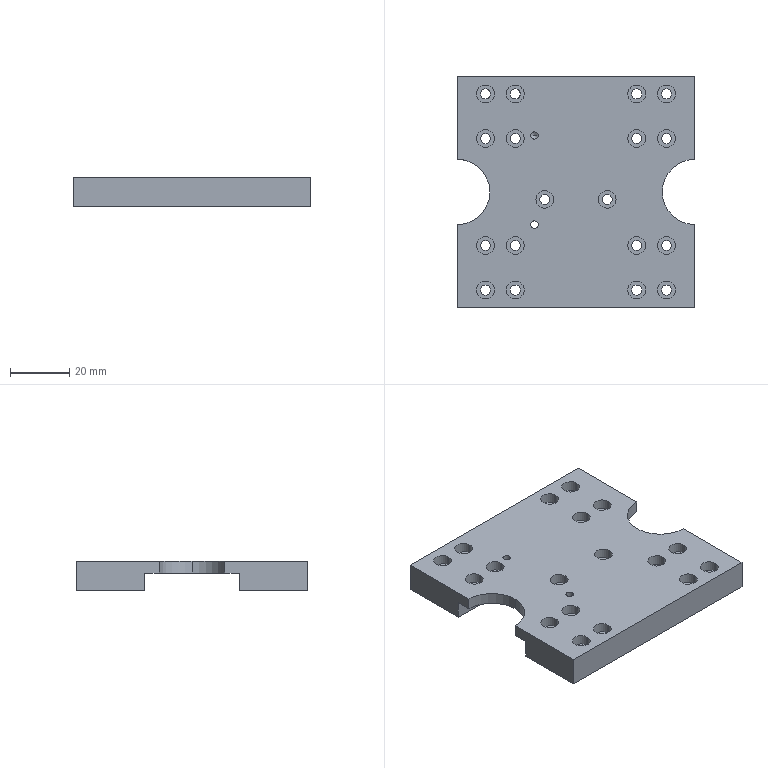Part | STEP file | 02-19 slide table plate | 1 solid | 119 faces | box 80 x 78 x 10 mm | volume 42678 mm3 | cylinder 83 | plane 30 | cone 6 | commonest cylinder face diameters 3.4 x36 6 x36 2.5 x8 22 x3